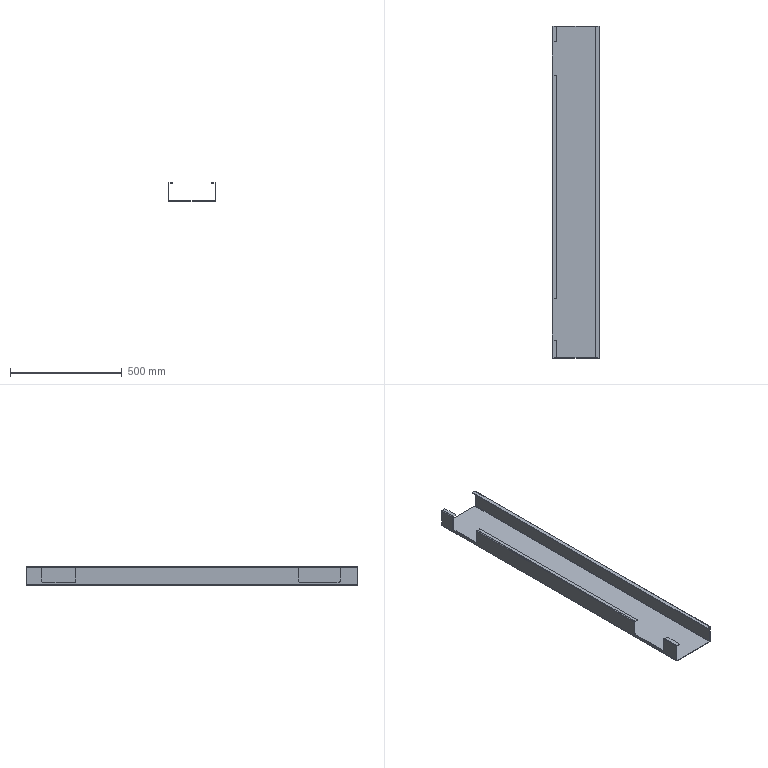Part | SolidWorks | features BaseBody 1 | 1 solid | 62 faces | box 214 x 1487 x 84 mm | volume 1444345 mm3 | plane 42 | cylinder 20 | commonest cylinder face diameters 10 x8 2 x6 7 x6